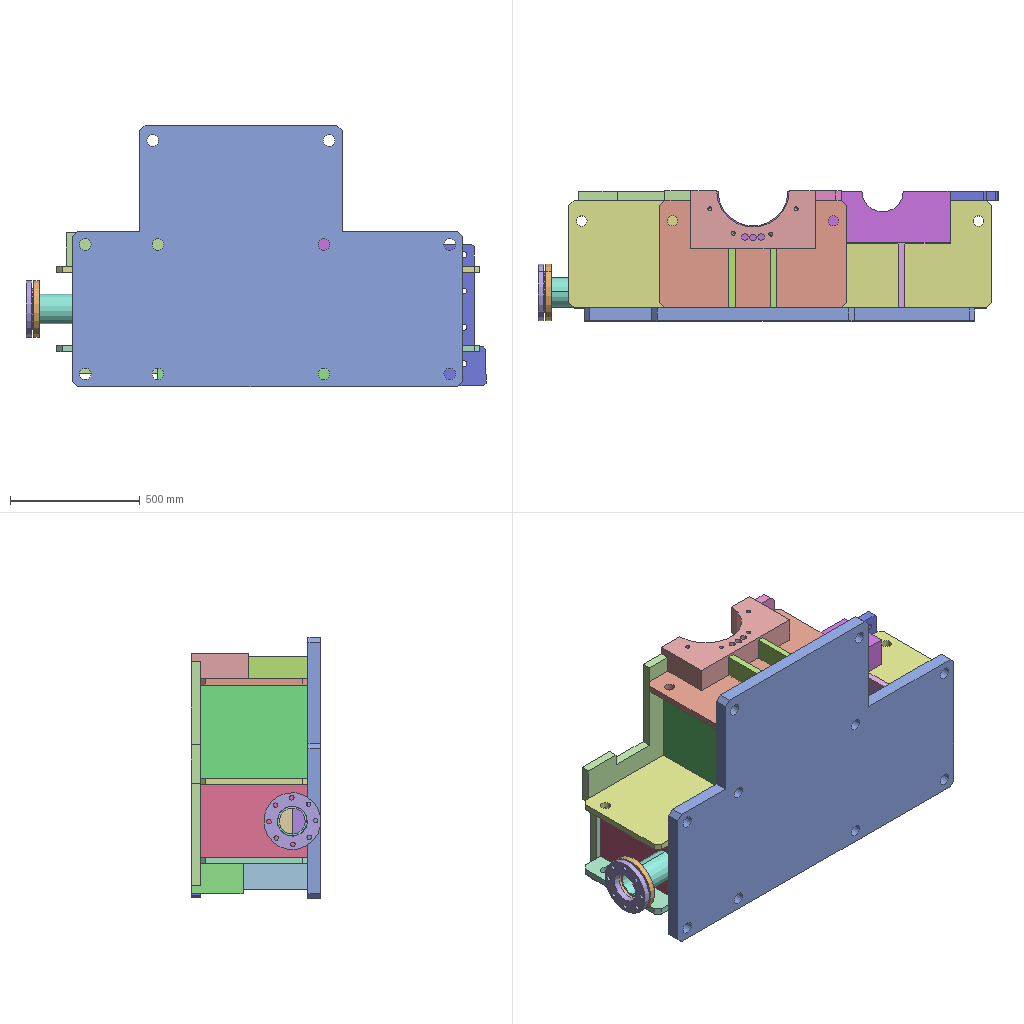Assembly | SolidWorks | 21 different items | 25 placed | box 1774 x 500 x 1010 mm
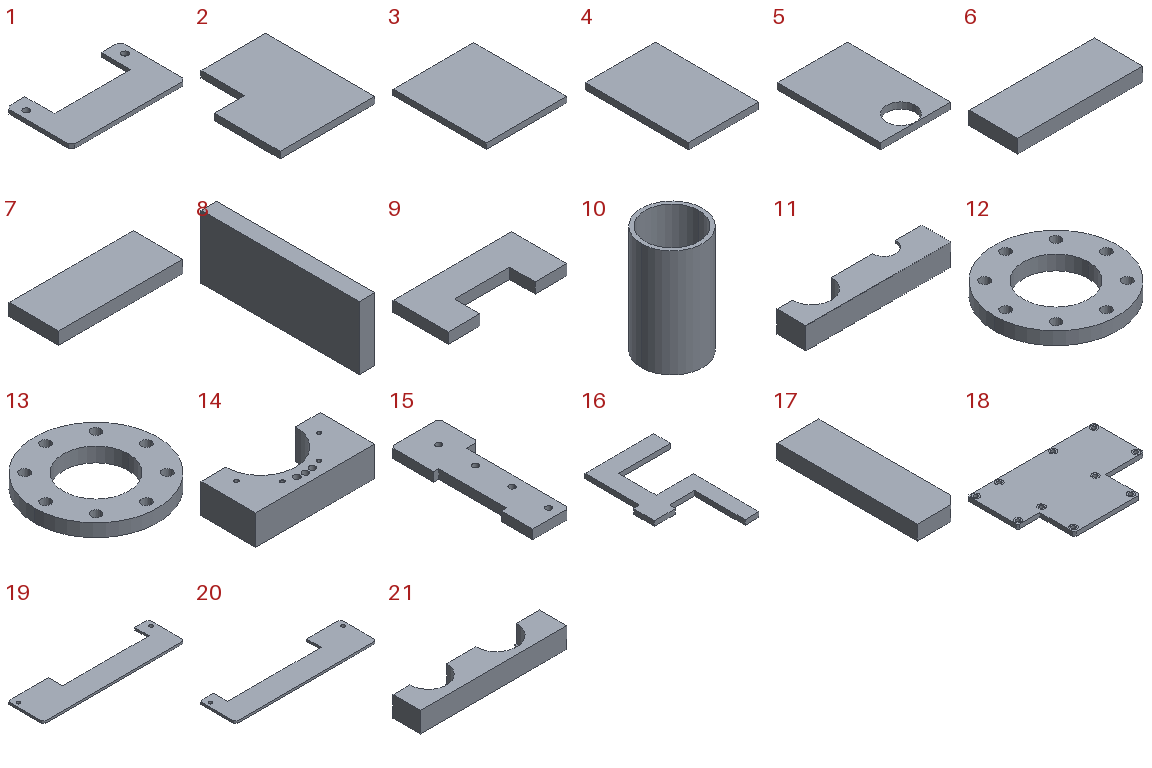Parts list (item | quantity | size | volume | features):
1 | x1 | 720 x 415 x 25 mm | 5167168 mm3 | features Chamfer 1, Extrusion 1
2 | x1 | 360 x 415 x 25 mm | 3260625 mm3 | features Extrusion 1
3 | x1 | 360 x 415 x 25 mm | 3735000 mm3 | features Extrusion 1
4 | x1 | 280 x 415 x 25 mm | 2905000 mm3 | features Extrusion 1
5 | x1 | 280 x 415 x 25 mm | 2640792 mm3 | features Extrusion 1
6 | x2 | 230 x 90 x 25 mm | 517500 mm3 | features Extrusion 1
7 | x1 | 250 x 100 x 25 mm | 625000 mm3 | features Extrusion 1
8 | x3 | 25 x 250 x 100 mm | 625000 mm3 | features Extrusion 1
9 | x2 | 280 x 130 x 25 mm | 715000 mm3 | features Extrusion 1
10 | x1 | 114 x 114 x 200 mm | 470611 mm3 | features Extrusion 1, RefAxis 1
11 | x1 | 1000 x 200 x 150 mm | 22425057 mm3 | features RefAxis 2, Chamfer 1, Extrusion 1, ICE 1, RevCut 1
12 | x1 | 220 x 220 x 26 mm | 615594 mm3 | features Extrusion 1, ICE 1, RefAxis 1, RevCut 1
13 | x1 | 220 x 220 x 26 mm | 615594 mm3 | features Extrusion 1, ICE 1, RevCut 1
14 | x1 | 480 x 220 x 120 mm | 8780124 mm3 | features ICE 2, Extrusion 1, HoleWzd 1, RefAxis 1
15 | x1 | 185 x 545 x 35 mm | 2664531 mm3 | features Chamfer 1, Extrusion 1, ICE 1
16 | x1 | 540 x 865 x 35 mm | 6369754 mm3 | features Extrusion 1
17 | x1 | 100 x 335 x 35 mm | 1165500 mm3 | features Chamfer 1, Extrusion 1
18 | x1 | 1505 x 1010 x 50 mm | 60216062 mm3 | features Chamfer 1, Extrusion 1, HoleWzd 1
19 | x1 | 1630 x 415 x 25 mm | 12703418 mm3 | features Chamfer 1, Extrusion 1, ICE 1
20 | x1 | 1630 x 415 x 25 mm | 12373418 mm3 | features Chamfer 1, Extrusion 1, ICE 1
21 | x1 | 1080 x 200 x 150 mm | 23020382 mm3 | features ICE 2, RefAxis 2, Extrusion 1
Mates (type | each side: item.copy, entity, surface, feature):
Parallel | 14.1 face plane Boss-Extrude1 | 18.1 face plane Boss-Extrude1
Coincident | 13.1 face plane Boss-Extrude1 | 12.1 face plane Boss-Extrude1
Concentric | 13.1 face cylinder Cut-Extrude1 | 12.1 face cylinder Cut-Extrude2
Concentric | 10.1 face cylinder Boss-Extrude1 | 13.1 face cylinder Cut-Extrude1
DistanceDim | 10.1 face plane Boss-Extrude1 | 13.1 face plane Boss-Extrude1
Coincident | 18.1 face plane Boss-Extrude1 | 6.1 face plane Boss-Extrude1
DistanceDim | 14.1 axis | 6.1 face plane Boss-Extrude1
Coincident | 14.1 face plane Boss-Extrude1 | 6.1 face plane Boss-Extrude1
Coincident | 14.1 face plane Boss-Extrude1 | 6.2 face plane Boss-Extrude1
Coincident | 18.1 face plane Boss-Extrude1 | 6.2 face plane Boss-Extrude1
DistanceDim | 14.1 axis | 6.2 face plane Boss-Extrude1
Coincident | 18.1 face plane Boss-Extrude1 | 5.1 face plane Boss-Extrude1
Parallel | 10.1 face plane Boss-Extrude1 | 5.1 face plane Boss-Extrude1
Coincident | 18.1 face plane Boss-Extrude1 | 8.1 face plane Boss-Extrude1
Coincident | 18.1 face plane Boss-Extrude1 | 8.2 face plane Boss-Extrude1
Coincident | 18.1 face plane Boss-Extrude1 | 8.3 face plane Boss-Extrude1
DistanceDim | 10.1 axis | 18.1 face plane Boss-Extrude1
Concentric | 13.1 face cylinder Boss-Extrude1 | 12.1 face cylinder Boss-Extrude1
Coincident | 18.1 face plane Boss-Extrude1 | 19.1 face plane Boss-Extrude1
Coincident | 18.1 face plane Boss-Extrude1 | 7.1 face plane Boss-Extrude1
DistanceDim | 6.1 face plane Boss-Extrude1 | 14.1 face plane Boss-Extrude1
DistanceDim | 14.1 face plane Boss-Extrude1 | 6.2 face plane Boss-Extrude1
DistanceDim | 14.1 axis | 18.1 face plane Boss-Extrude1
Coincident | 14.1 axis | 11.1 axis
Coincident | 21.1 axis | 11.1 axis | 2 times
DistanceDim | 19.1 face plane Boss-Extrude1 | 11.1 face plane Boss-Extrude1
Coincident | 7.1 face plane Boss-Extrude1 | 11.1 face plane Boss-Extrude1
Parallel | 7.1 face plane Boss-Extrude1 | 11.1 face plane Boss-Extrude1
Coincident | 7.1 face plane Boss-Extrude1 | 19.1 face plane Boss-Extrude1
Coincident | 18.1 face plane Boss-Extrude1 | 20.1 face plane Boss-Extrude1
DistanceDim | 20.1 face plane Boss-Extrude1 | 21.1 face plane Boss-Extrude1 | 2 times
Coincident | 8.3 face plane Boss-Extrude1 | 20.1 face plane Boss-Extrude1
Coincident | 8.2 face plane Boss-Extrude1 | 20.1 face plane Boss-Extrude1
Coincident | 8.1 face plane Boss-Extrude1 | 20.1 face plane Boss-Extrude1
Width | 19.1 face plane Boss-Extrude1 | 19.1 face plane Boss-Extrude1 | 20.1 face plane Boss-Extrude1 | 20.1 face plane Boss-Extrude1
Coincident | 14.1 face plane Boss-Extrude1 | 1.1 face plane Boss-Extrude1 | 2 times
Coincident | 18.1 face plane Boss-Extrude1 | 1.1 face plane Boss-Extrude1
DistanceDim | 21.1 face plane Boss-Extrude1 | 15.1 face plane Boss-Extrude1
DistanceDim | 15.1 face plane Boss-Extrude1 | 11.1 face plane Boss-Extrude1
DistanceDim | 10.1 axis | 15.1 face plane Boss-Extrude1
Coincident | 21.1 face plane Boss-Extrude1 | 15.1 face plane Boss-Extrude1
Coincident | 14.1 face plane Boss-Extrude1 | 16.1 face plane Boss-Extrude1 | 2 times
DistanceDim | 16.1 face plane Boss-Extrude1 | 14.1 face plane Boss-Extrude1
Coincident | 11.1 face plane Boss-Extrude1 | 17.1 face plane Boss-Extrude1
Coincident | 14.1 face plane Boss-Extrude1 | 17.1 face plane Boss-Extrude1 | 2 times
Parallel | 7.1 face plane Boss-Extrude1 | 2.1 face plane Boss-Extrude1
Coincident | 18.1 face plane Boss-Extrude1 | 2.1 face plane Boss-Extrude1
Coincident | 19.1 face plane Boss-Extrude1 | 2.1 face plane Boss-Extrude1
Coincident | 1.1 face plane Boss-Extrude1 | 2.1 face plane Boss-Extrude1
Coincident | 17.1 face plane Boss-Extrude1 | 2.1 face plane Boss-Extrude1
Coincident | 18.1 face plane Boss-Extrude1 | 9.1 face plane Boss-Extrude1
Coincident | 20.1 face plane Boss-Extrude1 | 9.1 face plane Boss-Extrude1
Coincident | 19.1 face plane Boss-Extrude1 | 9.1 face plane Boss-Extrude1
Coincident | 5.1 face plane Boss-Extrude1 | 20.1 face plane Boss-Extrude1
Coincident | 20.1 face plane Boss-Extrude1 | 9.2 face plane Boss-Extrude1
Coincident | 18.1 face plane Boss-Extrude1 | 9.2 face plane Boss-Extrude1
DistanceDim | 9.2 face plane Boss-Extrude1 | 15.1 face plane Boss-Extrude1
DistanceDim | 11.1 axis | 9.1 face plane Boss-Extrude1
Coincident | 19.1 face plane Boss-Extrude1 | 3.1 face plane Boss-Extrude1
Coincident | 18.1 face plane Boss-Extrude1 | 3.1 face plane Boss-Extrude1
Coincident | 11.1 face plane Boss-Extrude1 | 3.1 face plane Boss-Extrude1
DistanceDim | 5.1 face plane Boss-Extrude1 | 10.1 face plane Boss-Extrude1
DistanceDim | 14.1 axis | 13.1 face plane Cut-Revolve1
Tangent | 18.1 face plane Boss-Extrude1 | 13.1 face cylinder Boss-Extrude1
Coincident | 18.1 face plane Boss-Extrude1 | 4.1 face plane Boss-Extrude1
Coincident | 20.1 face plane Boss-Extrude1 | 4.1 face plane Boss-Extrude1
Coincident | 15.1 face plane Boss-Extrude1 | 4.1 face plane Boss-Extrude1